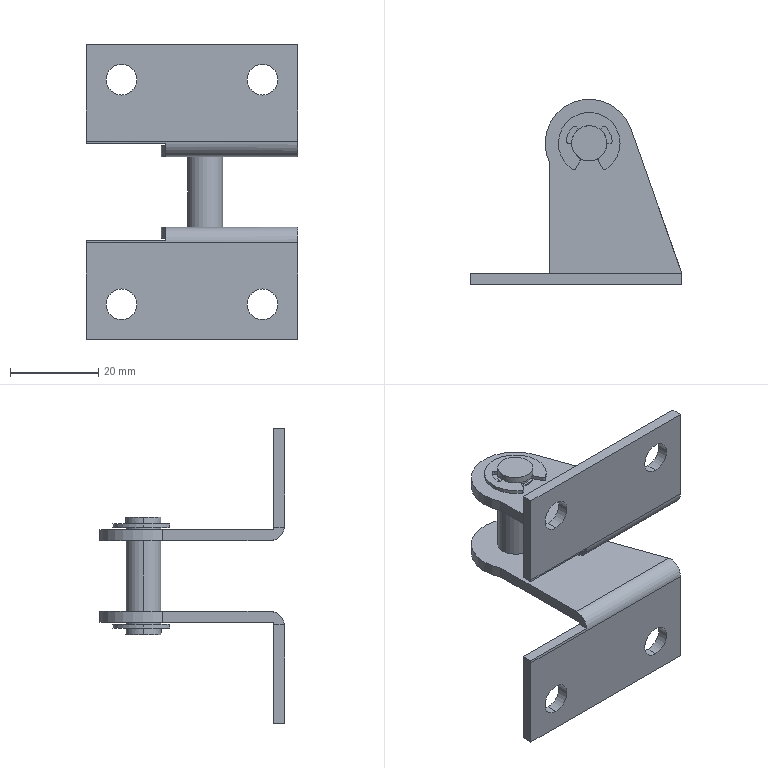Part | SolidWorks | features BaseBody 1 | 1 solid | 96 faces | box 48 x 42 x 67 mm | volume 10967 mm3 | cylinder 50 | plane 46 | commonest cylinder face diameters 1 x14 7 x14 8 x10 14 x6 10.5 x4 20 x2